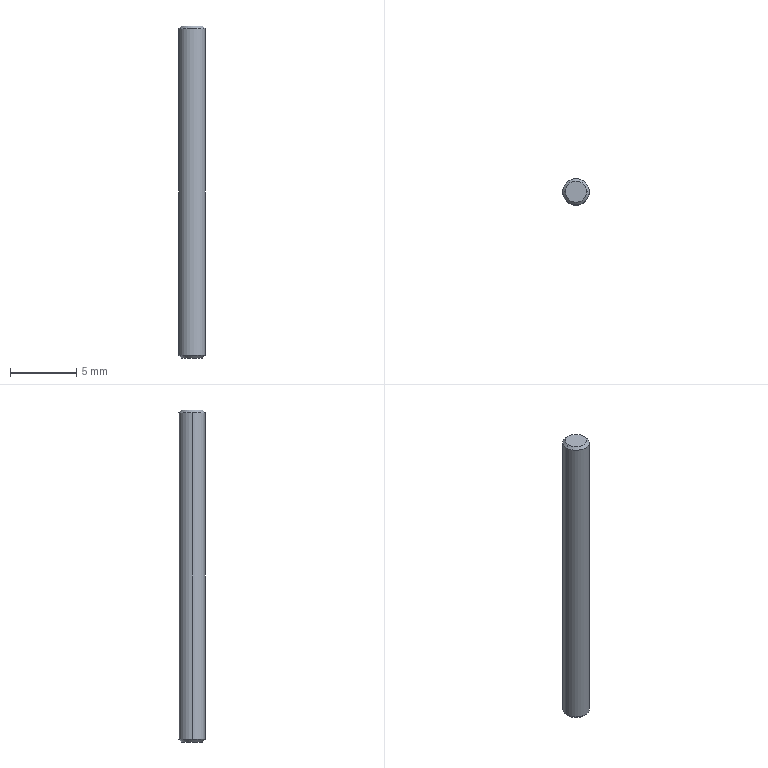Part | SolidWorks | features RefAxis 3, 3DProfileFeature 1, Revolution 1 | 1 solid | 8 faces | box 2 x 2 x 25 mm | volume 78.305 mm3 | cone 4 | cylinder 2 | plane 2 | commonest cylinder face diameters 2 x2
STEP:
#1=CARTESIAN_POINT('',(-0.8,0.,0.));
#2=VERTEX_POINT('',#1);
#3=CARTESIAN_POINT('',(0.8,0.,0.));
#4=VERTEX_POINT('',#3);
#5=CARTESIAN_POINT('',(0.,0.,0.));
#6=DIRECTION('',(0.,0.,-1.));
#7=DIRECTION('',(-1.,0.,0.));
#8=AXIS2_PLACEMENT_3D('',#5,#6,#7);
#9=CIRCLE('',#8,0.8);
#10=EDGE_CURVE('',#2,#4,#9,.T.);
#11=ORIENTED_EDGE('',*,*,#10,.T.);
#12=CARTESIAN_POINT('',(1.,0.,-0.2));
#13=VERTEX_POINT('',#12);
#14=CARTESIAN_POINT('',(0.8,0.,0.));
#15=DIRECTION('',(0.7071,0.,-0.7071));
#16=VECTOR('',#15,1000.);
#17=LINE('',#14,#16);
#18=EDGE_CURVE('',#4,#13,#17,.T.);
#19=ORIENTED_EDGE('',*,*,#18,.T.);
#20=CARTESIAN_POINT('',(-1.,0.,-0.2));
#21=VERTEX_POINT('',#20);
#22=CARTESIAN_POINT('',(0.,0.,-0.2));
#23=DIRECTION('',(0.,0.,-1.));
#24=DIRECTION('',(-1.,0.,0.));
#25=AXIS2_PLACEMENT_3D('',#22,#23,#24);
#26=CIRCLE('',#25,1.);
#27=EDGE_CURVE('',#21,#13,#26,.T.);
#28=ORIENTED_EDGE('',*,*,#27,.F.);
#29=CARTESIAN_POINT('',(-0.8,0.,0.));
#30=DIRECTION('',(-0.7071,0.,-0.7071));
#31=VECTOR('',#30,1000.);
#32=LINE('',#29,#31);
#33=EDGE_CURVE('',#2,#21,#32,.T.);
#34=ORIENTED_EDGE('',*,*,#33,.F.);
#35=EDGE_LOOP('',(#11,#19,#28,#34));
#36=FACE_OUTER_BOUND('',#35,.T.);
#37=CARTESIAN_POINT('',(0.,0.,0.));
#38=DIRECTION('',(0.,0.,-1.));
#39=DIRECTION('',(-1.,0.,0.));
#40=AXIS2_PLACEMENT_3D('',#37,#38,#39);
#41=CONICAL_SURFACE('',#40,0.8,0.7854);
#42=ADVANCED_FACE('',(#36),#41,.T.);
#43=ORIENTED_EDGE('',*,*,#27,.T.);
#44=CARTESIAN_POINT('',(1.,0.,-24.8));
#45=VERTEX_POINT('',#44);
#46=CARTESIAN_POINT('',(1.,0.,0.));
#47=DIRECTION('',(0.,0.,-1.));
#48=VECTOR('',#47,1000.);
#49=LINE('',#46,#48);
#50=EDGE_CURVE('',#13,#45,#49,.T.);
#51=ORIENTED_EDGE('',*,*,#50,.T.);
#52=CARTESIAN_POINT('',(-1.,0.,-24.8));
#53=VERTEX_POINT('',#52);
#54=CARTESIAN_POINT('',(0.,0.,-24.8));
#55=DIRECTION('',(0.,0.,-1.));
#56=DIRECTION('',(-1.,0.,0.));
#57=AXIS2_PLACEMENT_3D('',#54,#55,#56);
#58=CIRCLE('',#57,1.);
#59=EDGE_CURVE('',#53,#45,#58,.T.);
#60=ORIENTED_EDGE('',*,*,#59,.F.);
#61=CARTESIAN_POINT('',(-1.,0.,0.));
#62=DIRECTION('',(0.,0.,-1.));
#63=VECTOR('',#62,1000.);
#64=LINE('',#61,#63);
#65=EDGE_CURVE('',#21,#53,#64,.T.);
#66=ORIENTED_EDGE('',*,*,#65,.F.);
#67=EDGE_LOOP('',(#43,#51,#60,#66));
#68=FACE_OUTER_BOUND('',#67,.T.);
#69=CARTESIAN_POINT('',(0.,0.,0.));
#70=DIRECTION('',(0.,0.,-1.));
#71=DIRECTION('',(-1.,0.,0.));
#72=AXIS2_PLACEMENT_3D('',#69,#70,#71);
#73=CYLINDRICAL_SURFACE('',#72,1.);
#74=ADVANCED_FACE('',(#68),#73,.T.);
#75=CARTESIAN_POINT('',(-0.8,0.,-25.));
#76=VERTEX_POINT('',#75);
#77=CARTESIAN_POINT('',(0.8,0.,-25.));
#78=VERTEX_POINT('',#77);
#79=CARTESIAN_POINT('',(0.,0.,-25.));
#80=DIRECTION('',(0.,0.,-1.));
#81=DIRECTION('',(-1.,0.,0.));
#82=AXIS2_PLACEMENT_3D('',#79,#80,#81);
#83=CIRCLE('',#82,0.8);
#84=EDGE_CURVE('',#76,#78,#83,.T.);
#85=ORIENTED_EDGE('',*,*,#84,.F.);
#86=CARTESIAN_POINT('',(-1.,0.,-24.8));
#87=DIRECTION('',(-0.7071,0.,0.7071));
#88=VECTOR('',#87,1000.);
#89=LINE('',#86,#88);
#90=EDGE_CURVE('',#76,#53,#89,.T.);
#91=ORIENTED_EDGE('',*,*,#90,.T.);
#92=ORIENTED_EDGE('',*,*,#59,.T.);
#93=CARTESIAN_POINT('',(1.,0.,-24.8));
#94=DIRECTION('',(0.7071,0.,0.7071));
#95=VECTOR('',#94,1000.);
#96=LINE('',#93,#95);
#97=EDGE_CURVE('',#78,#45,#96,.T.);
#98=ORIENTED_EDGE('',*,*,#97,.F.);
#99=EDGE_LOOP('',(#85,#91,#92,#98));
#100=FACE_OUTER_BOUND('',#99,.T.);
#101=CARTESIAN_POINT('',(0.,0.,-24.8));
#102=DIRECTION('',(0.,0.,1.));
#103=DIRECTION('',(1.,0.,0.));
#104=AXIS2_PLACEMENT_3D('',#101,#102,#103);
#105=CONICAL_SURFACE('',#104,1.,0.7854);
#106=ADVANCED_FACE('',(#100),#105,.T.);
#107=CARTESIAN_POINT('',(0.,0.,-25.));
#108=DIRECTION('',(0.,0.,-1.));
#109=DIRECTION('',(-1.,0.,0.));
#110=AXIS2_PLACEMENT_3D('',#107,#108,#109);
#111=CIRCLE('',#110,0.8);
#112=EDGE_CURVE('',#78,#76,#111,.T.);
#113=ORIENTED_EDGE('',*,*,#112,.T.);
#114=ORIENTED_EDGE('',*,*,#84,.T.);
#115=EDGE_LOOP('',(#113,#114));
#116=FACE_OUTER_BOUND('',#115,.T.);
#117=CARTESIAN_POINT('',(0.,0.,-25.));
#118=DIRECTION('',(0.,0.,1.));
#119=DIRECTION('',(1.,0.,0.));
#120=AXIS2_PLACEMENT_3D('',#117,#118,#119);
#121=PLANE('',#120);
#122=ADVANCED_FACE('',(#116),#121,.F.);
#123=ORIENTED_EDGE('',*,*,#90,.F.);
#124=ORIENTED_EDGE('',*,*,#112,.F.);
#125=ORIENTED_EDGE('',*,*,#97,.T.);
#126=CARTESIAN_POINT('',(0.,0.,-24.8));
#127=DIRECTION('',(0.,0.,-1.));
#128=DIRECTION('',(-1.,0.,0.));
#129=AXIS2_PLACEMENT_3D('',#126,#127,#128);
#130=CIRCLE('',#129,1.);
#131=EDGE_CURVE('',#45,#53,#130,.T.);
#132=ORIENTED_EDGE('',*,*,#131,.T.);
#133=EDGE_LOOP('',(#123,#124,#125,#132));
#134=FACE_OUTER_BOUND('',#133,.T.);
#135=CARTESIAN_POINT('',(0.,0.,-24.8));
#136=DIRECTION('',(0.,0.,1.));
#137=DIRECTION('',(1.,0.,0.));
#138=AXIS2_PLACEMENT_3D('',#135,#136,#137);
#139=CONICAL_SURFACE('',#138,1.,0.7854);
#140=ADVANCED_FACE('',(#134),#139,.T.);
#141=ORIENTED_EDGE('',*,*,#50,.F.);
#142=CARTESIAN_POINT('',(0.,0.,-0.2));
#143=DIRECTION('',(0.,0.,-1.));
#144=DIRECTION('',(-1.,0.,0.));
#145=AXIS2_PLACEMENT_3D('',#142,#143,#144);
#146=CIRCLE('',#145,1.);
#147=EDGE_CURVE('',#13,#21,#146,.T.);
#148=ORIENTED_EDGE('',*,*,#147,.T.);
#149=ORIENTED_EDGE('',*,*,#65,.T.);
#150=ORIENTED_EDGE('',*,*,#131,.F.);
#151=EDGE_LOOP('',(#141,#148,#149,#150));
#152=FACE_OUTER_BOUND('',#151,.T.);
#153=CARTESIAN_POINT('',(0.,0.,0.));
#154=DIRECTION('',(0.,0.,-1.));
#155=DIRECTION('',(-1.,0.,0.));
#156=AXIS2_PLACEMENT_3D('',#153,#154,#155);
#157=CYLINDRICAL_SURFACE('',#156,1.);
#158=ADVANCED_FACE('',(#152),#157,.T.);
#159=ORIENTED_EDGE('',*,*,#18,.F.);
#160=CARTESIAN_POINT('',(0.,0.,0.));
#161=DIRECTION('',(0.,0.,-1.));
#162=DIRECTION('',(-1.,0.,0.));
#163=AXIS2_PLACEMENT_3D('',#160,#161,#162);
#164=CIRCLE('',#163,0.8);
#165=EDGE_CURVE('',#4,#2,#164,.T.);
#166=ORIENTED_EDGE('',*,*,#165,.T.);
#167=ORIENTED_EDGE('',*,*,#33,.T.);
#168=ORIENTED_EDGE('',*,*,#147,.F.);
#169=EDGE_LOOP('',(#159,#166,#167,#168));
#170=FACE_OUTER_BOUND('',#169,.T.);
#171=CARTESIAN_POINT('',(0.,0.,0.));
#172=DIRECTION('',(0.,0.,-1.));
#173=DIRECTION('',(-1.,0.,0.));
#174=AXIS2_PLACEMENT_3D('',#171,#172,#173);
#175=CONICAL_SURFACE('',#174,0.8,0.7854);
#176=ADVANCED_FACE('',(#170),#175,.T.);
#177=ORIENTED_EDGE('',*,*,#10,.F.);
#178=ORIENTED_EDGE('',*,*,#165,.F.);
#179=EDGE_LOOP('',(#177,#178));
#180=FACE_OUTER_BOUND('',#179,.T.);
#181=CARTESIAN_POINT('',(0.8,0.,0.));
#182=DIRECTION('',(0.,0.,-1.));
#183=DIRECTION('',(-1.,0.,0.));
#184=AXIS2_PLACEMENT_3D('',#181,#182,#183);
#185=PLANE('',#184);
#186=ADVANCED_FACE('',(#180),#185,.F.);
#187=CLOSED_SHELL('',(#42,#74,#106,#122,#140,#158,#176,#186));
#188=MANIFOLD_SOLID_BREP('',#187);
#189=CARTESIAN_POINT('',(0.,0.,0.));
#190=DIRECTION('',(0.,0.,1.));
#191=DIRECTION('',(1.,0.,0.));
#192=AXIS2_PLACEMENT_3D('',#189,#190,#191);
#193=(LENGTH_UNIT()NAMED_UNIT(*)SI_UNIT(.MILLI.,.METRE.));
#194=UNCERTAINTY_MEASURE_WITH_UNIT(LENGTH_MEASURE(0.00001),#193,'','');
#195=(NAMED_UNIT(*)PLANE_ANGLE_UNIT()SI_UNIT($,.RADIAN.));
#196=(NAMED_UNIT(*)SI_UNIT($,.STERADIAN.)SOLID_ANGLE_UNIT());
#197=(GEOMETRIC_REPRESENTATION_CONTEXT(3)GLOBAL_UNCERTAINTY_ASSIGNED_CONTEXT((#194))GLOBAL_UNIT_ASSIGNED_CONTEXT((#193,#195,#196))REPRESENTATION_CONTEXT('',''));
#198=ADVANCED_BREP_SHAPE_REPRESENTATION('',(#188,#192),#197);